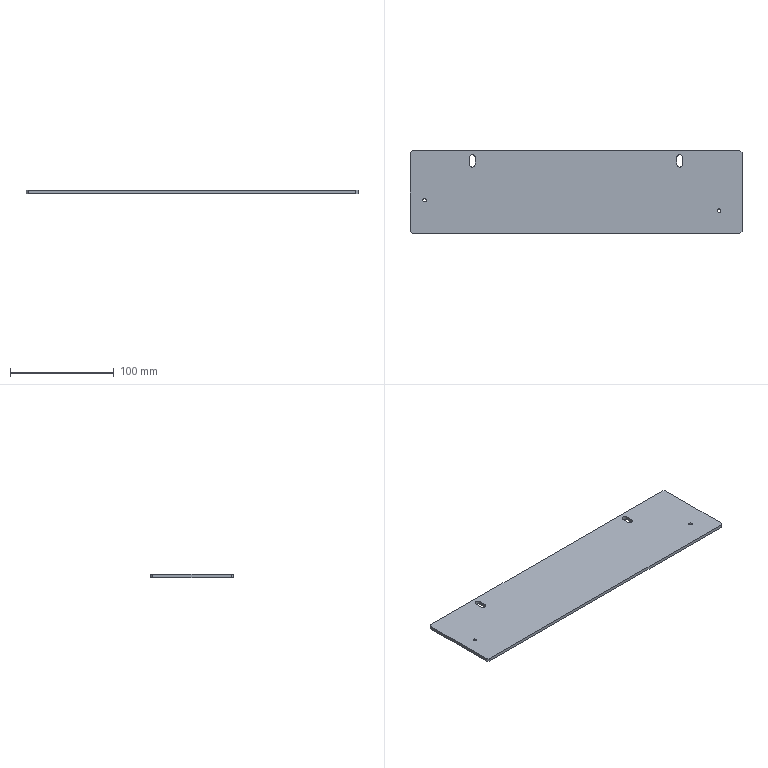Part | STEP file | power strip mounting plate | 1 solid | 22 faces | box 320 x 80 x 3 mm | volume 76368 mm3 | plane 14 | cylinder 8 | commonest cylinder face diameters 3.3 x4 5.5 x4